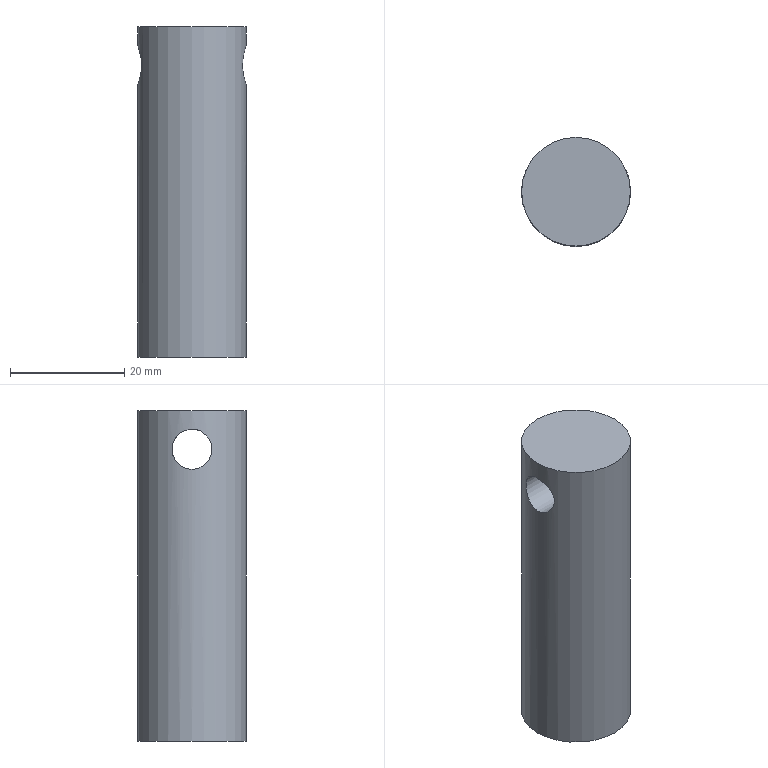Part | NX | features solid 2 | 1 solid | 4 faces | box 19 x 19 x 57.7 mm | volume 15641 mm3 | cylinder 2 | plane 2 | commonest cylinder face diameters 7 x1 19 x1
STEP:
#1=CARTESIAN_POINT('',(-1549.5,415.,19.5));
#2=VERTEX_POINT('',#1);
#3=CARTESIAN_POINT('',(-1549.178,417.742,18.743));
#4=CARTESIAN_POINT('',(-1549.661,415.001,19.879));
#5=CARTESIAN_POINT('',(-1549.178,412.255,18.74));
#6=CARTESIAN_POINT('',(-1548.659,411.121,16.005));
#7=CARTESIAN_POINT('',(-1549.178,412.258,13.256));
#8=CARTESIAN_POINT('',(-1549.661,414.997,12.122));
#9=CARTESIAN_POINT('',(-1549.178,417.745,13.258));
#10=CARTESIAN_POINT('',(-1548.659,418.878,16.001));
#11=CARTESIAN_POINT('',(-1549.178,417.742,18.743));
#12=CARTESIAN_POINT('',(-1549.661,415.001,19.879));
#13=CARTESIAN_POINT('',(-1549.178,412.255,18.74));
#14=B_SPLINE_CURVE_WITH_KNOTS('',3,(#3,#4,#5,#6,#7,#8,#9,#10,#11,#12,#13),.UNSPECIFIED.,.T.,.F.,(1,1,1,1,1,1,1,1,1,1,1,1,1,1,1),(-0.00828,-0.00552,-0.00276,0.,0.00276,0.00552,0.00828,0.01104,0.0138,0.01656,0.01932,0.02208,0.02484,0.0276,0.03036),.UNSPECIFIED.);
#15=EDGE_CURVE('',#2,#2,#14,.T.);
#16=ORIENTED_EDGE('',*,*,#15,.T.);
#17=EDGE_LOOP('',(#16));
#18=FACE_BOUND('',#17,.T.);
#19=CARTESIAN_POINT('',(-1530.5,415.,12.5));
#20=VERTEX_POINT('',#19);
#21=CARTESIAN_POINT('',(-1530.822,417.742,13.257));
#22=CARTESIAN_POINT('',(-1530.339,415.001,12.121));
#23=CARTESIAN_POINT('',(-1530.822,412.255,13.26));
#24=CARTESIAN_POINT('',(-1531.341,411.121,15.995));
#25=CARTESIAN_POINT('',(-1530.822,412.258,18.744));
#26=CARTESIAN_POINT('',(-1530.339,414.997,19.878));
#27=CARTESIAN_POINT('',(-1530.822,417.745,18.742));
#28=CARTESIAN_POINT('',(-1531.341,418.878,15.999));
#29=CARTESIAN_POINT('',(-1530.822,417.742,13.257));
#30=CARTESIAN_POINT('',(-1530.339,415.001,12.121));
#31=CARTESIAN_POINT('',(-1530.822,412.255,13.26));
#32=B_SPLINE_CURVE_WITH_KNOTS('',3,(#21,#22,#23,#24,#25,#26,#27,#28,#29,#30,#31),.UNSPECIFIED.,.T.,.F.,(1,1,1,1,1,1,1,1,1,1,1,1,1,1,1),(-0.00828,-0.00552,-0.00276,0.,0.00276,0.00552,0.00828,0.01104,0.0138,0.01656,0.01932,0.02208,0.02484,0.0276,0.03036),.UNSPECIFIED.);
#33=EDGE_CURVE('',#20,#20,#32,.T.);
#34=ORIENTED_EDGE('',*,*,#33,.T.);
#35=EDGE_LOOP('',(#34));
#36=FACE_BOUND('',#35,.T.);
#37=CARTESIAN_POINT('',(-1530.5,415.,22.7));
#38=VERTEX_POINT('',#37);
#39=CARTESIAN_POINT('',(-1540.,415.,22.7));
#40=DIRECTION('',(0.,0.,1.));
#41=DIRECTION('',(1.,0.,0.));
#42=AXIS2_PLACEMENT_3D('',#39,#40,#41);
#43=CIRCLE('',#42,9.5);
#44=EDGE_CURVE('',#38,#38,#43,.T.);
#45=ORIENTED_EDGE('',*,*,#44,.F.);
#46=EDGE_LOOP('',(#45));
#47=FACE_BOUND('',#46,.T.);
#48=CARTESIAN_POINT('',(-1540.,424.5,-35.));
#49=VERTEX_POINT('',#48);
#50=CARTESIAN_POINT('',(-1540.,415.,-35.));
#51=DIRECTION('',(0.,0.,-1.));
#52=DIRECTION('',(0.,1.,0.));
#53=AXIS2_PLACEMENT_3D('',#50,#51,#52);
#54=CIRCLE('',#53,9.5);
#55=EDGE_CURVE('',#49,#49,#54,.F.);
#56=ORIENTED_EDGE('',*,*,#55,.T.);
#57=EDGE_LOOP('',(#56));
#58=FACE_BOUND('',#57,.T.);
#59=CARTESIAN_POINT('',(-1540.,415.,22.7));
#60=DIRECTION('',(0.,0.,-1.));
#61=DIRECTION('',(-1.,0.,0.));
#62=AXIS2_PLACEMENT_3D('',#59,#60,#61);
#63=CYLINDRICAL_SURFACE('',#62,9.5);
#64=ADVANCED_FACE('',(#18,#36,#47,#58),#63,.T.);
#65=ORIENTED_EDGE('',*,*,#44,.T.);
#66=EDGE_LOOP('',(#65));
#67=FACE_BOUND('',#66,.T.);
#68=CARTESIAN_POINT('',(-1540.,415.,22.7));
#69=DIRECTION('',(0.,0.,1.));
#70=DIRECTION('',(1.,0.,0.));
#71=AXIS2_PLACEMENT_3D('',#68,#69,#70);
#72=PLANE('',#71);
#73=ADVANCED_FACE('',(#67),#72,.T.);
#74=ORIENTED_EDGE('',*,*,#55,.F.);
#75=EDGE_LOOP('',(#74));
#76=FACE_BOUND('',#75,.T.);
#77=CARTESIAN_POINT('',(-1459.619,392.91,-35.));
#78=DIRECTION('',(0.,0.,-1.));
#79=DIRECTION('',(0.,1.,0.));
#80=AXIS2_PLACEMENT_3D('',#77,#78,#79);
#81=PLANE('',#80);
#82=ADVANCED_FACE('',(#76),#81,.T.);
#83=ORIENTED_EDGE('',*,*,#33,.F.);
#84=EDGE_LOOP('',(#83));
#85=FACE_BOUND('',#84,.T.);
#86=ORIENTED_EDGE('',*,*,#15,.F.);
#87=EDGE_LOOP('',(#86));
#88=FACE_BOUND('',#87,.T.);
#89=CARTESIAN_POINT('',(-1554.,415.,16.));
#90=DIRECTION('',(1.,0.,0.));
#91=DIRECTION('',(0.,0.,-1.));
#92=AXIS2_PLACEMENT_3D('',#89,#90,#91);
#93=CYLINDRICAL_SURFACE('',#92,3.5);
#94=ADVANCED_FACE('',(#85,#88),#93,.F.);
#95=CLOSED_SHELL('',(#64,#73,#82,#94));
#96=MANIFOLD_SOLID_BREP('',#95);
#97=(LENGTH_UNIT()NAMED_UNIT(*)SI_UNIT(.MILLI.,.METRE.));
#98=UNCERTAINTY_MEASURE_WITH_UNIT(LENGTH_MEASURE(0.0508),#97,'','');
#99=(NAMED_UNIT(*)PLANE_ANGLE_UNIT()SI_UNIT($,.RADIAN.));
#100=(NAMED_UNIT(*)SI_UNIT($,.STERADIAN.)SOLID_ANGLE_UNIT());
#101=(GEOMETRIC_REPRESENTATION_CONTEXT(3)GLOBAL_UNCERTAINTY_ASSIGNED_CONTEXT((#98))GLOBAL_UNIT_ASSIGNED_CONTEXT((#97,#99,#100))REPRESENTATION_CONTEXT('',''));
#102=ADVANCED_BREP_SHAPE_REPRESENTATION('',(#96),#101);